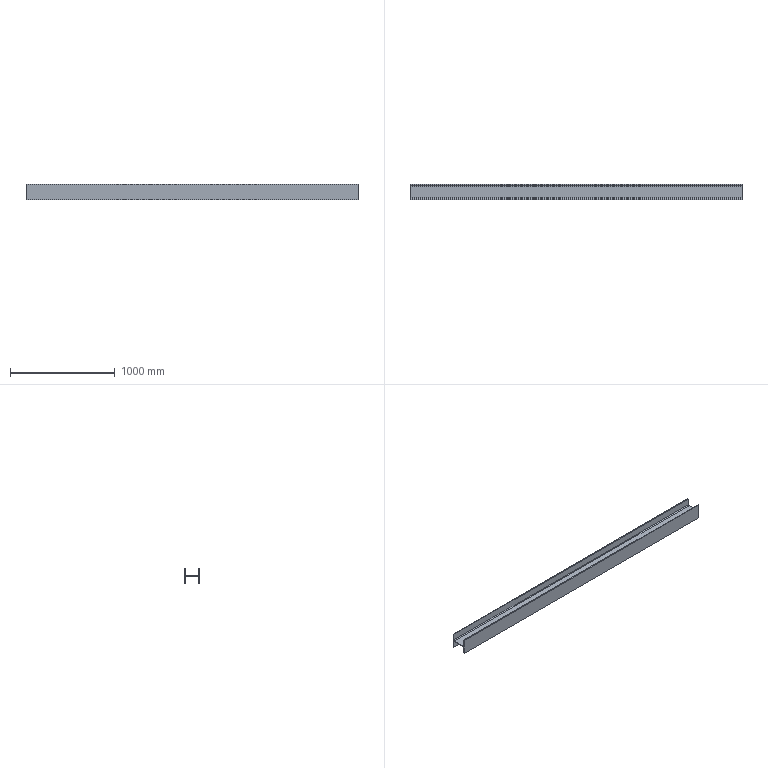Part | STEP file | 01-Cross beam H150X150_default<machining> | 1 solid | 18 faces | box 3170 x 150 x 150 mm | volume 12568854 mm3 | plane 14 | cylinder 4 | commonest cylinder face diameters 16 x4
STEP:
#1=CARTESIAN_POINT('',(0.,0.,0.));
#2=DIRECTION('',(0.,0.,1.));
#3=DIRECTION('',(1.,0.,0.));
#4=AXIS2_PLACEMENT_3D('',#1,#2,#3);
#5=CARTESIAN_POINT('',(0.,75.,75.));
#6=VERTEX_POINT('',#5);
#7=CARTESIAN_POINT('',(0.,65.,75.));
#8=VERTEX_POINT('',#7);
#9=CARTESIAN_POINT('',(0.,75.,75.));
#10=DIRECTION('',(0.,-1.,0.));
#11=VECTOR('',#10,1.);
#12=LINE('',#9,#11);
#13=CARTESIAN_POINT('',(3170.,75.,75.));
#14=DIRECTION('',(0.,0.,-1.));
#15=DIRECTION('',(0.,1.,0.));
#16=AXIS2_PLACEMENT_3D('',#13,#14,#15);
#17=PLANE('',#16);
#18=CARTESIAN_POINT('',(0.,-3170.));
#19=DIRECTION('',(-1.,0.));
#20=VECTOR('',#19,1.);
#21=LINE('',#18,#20);
#22=(GEOMETRIC_REPRESENTATION_CONTEXT(2)PARAMETRIC_REPRESENTATION_CONTEXT()REPRESENTATION_CONTEXT('',''));
#23=DEFINITIONAL_REPRESENTATION('',(#21),#22);
#24=PCURVE('',#17,#23);
#25=CARTESIAN_POINT('',(0.,57.,11.5));
#26=DIRECTION('',(1.,0.,0.));
#27=DIRECTION('',(0.,0.,-1.));
#28=AXIS2_PLACEMENT_3D('',#25,#26,#27);
#29=PLANE('',#28);
#30=CARTESIAN_POINT('',(-63.5,18.));
#31=DIRECTION('',(0.,-1.));
#32=VECTOR('',#31,1.);
#33=LINE('',#30,#32);
#34=(GEOMETRIC_REPRESENTATION_CONTEXT(2)PARAMETRIC_REPRESENTATION_CONTEXT()REPRESENTATION_CONTEXT('',''));
#35=DEFINITIONAL_REPRESENTATION('',(#33),#34);
#36=PCURVE('',#29,#35);
#37=SURFACE_CURVE('',#12,(#24,#36),.PCURVE_S1.);
#38=EDGE_CURVE('',#6,#8,#37,.T.);
#39=ORIENTED_EDGE('',*,*,#38,.T.);
#40=CARTESIAN_POINT('',(3170.,65.,75.));
#41=VERTEX_POINT('',#40);
#42=CARTESIAN_POINT('',(3170.,65.,75.));
#43=DIRECTION('',(-1.,0.,0.));
#44=VECTOR('',#43,1.);
#45=LINE('',#42,#44);
#46=CARTESIAN_POINT('',(-10.,0.));
#47=DIRECTION('',(0.,-1.));
#48=VECTOR('',#47,1.);
#49=LINE('',#46,#48);
#50=(GEOMETRIC_REPRESENTATION_CONTEXT(2)PARAMETRIC_REPRESENTATION_CONTEXT()REPRESENTATION_CONTEXT('',''));
#51=DEFINITIONAL_REPRESENTATION('',(#49),#50);
#52=PCURVE('',#17,#51);
#53=CARTESIAN_POINT('',(3170.,65.,75.));
#54=DIRECTION('',(0.,1.,0.));
#55=DIRECTION('',(0.,0.,1.));
#56=AXIS2_PLACEMENT_3D('',#53,#54,#55);
#57=PLANE('',#56);
#58=CARTESIAN_POINT('',(0.,0.));
#59=DIRECTION('',(0.,-1.));
#60=VECTOR('',#59,1.);
#61=LINE('',#58,#60);
#62=(GEOMETRIC_REPRESENTATION_CONTEXT(2)PARAMETRIC_REPRESENTATION_CONTEXT()REPRESENTATION_CONTEXT('',''));
#63=DEFINITIONAL_REPRESENTATION('',(#61),#62);
#64=PCURVE('',#57,#63);
#65=SURFACE_CURVE('',#45,(#52,#64),.PCURVE_S1.);
#66=EDGE_CURVE('',#41,#8,#65,.T.);
#67=ORIENTED_EDGE('',*,*,#66,.F.);
#68=CARTESIAN_POINT('',(3170.,75.,75.));
#69=VERTEX_POINT('',#68);
#70=CARTESIAN_POINT('',(3170.,75.,75.));
#71=DIRECTION('',(0.,-1.,0.));
#72=VECTOR('',#71,1.);
#73=LINE('',#70,#72);
#74=CARTESIAN_POINT('',(0.,0.));
#75=DIRECTION('',(-1.,0.));
#76=VECTOR('',#75,1.);
#77=LINE('',#74,#76);
#78=(GEOMETRIC_REPRESENTATION_CONTEXT(2)PARAMETRIC_REPRESENTATION_CONTEXT()REPRESENTATION_CONTEXT('',''));
#79=DEFINITIONAL_REPRESENTATION('',(#77),#78);
#80=PCURVE('',#17,#79);
#81=CARTESIAN_POINT('',(3170.,57.,11.5));
#82=DIRECTION('',(1.,0.,0.));
#83=DIRECTION('',(0.,0.,-1.));
#84=AXIS2_PLACEMENT_3D('',#81,#82,#83);
#85=PLANE('',#84);
#86=CARTESIAN_POINT('',(-63.5,18.));
#87=DIRECTION('',(0.,-1.));
#88=VECTOR('',#87,1.);
#89=LINE('',#86,#88);
#90=(GEOMETRIC_REPRESENTATION_CONTEXT(2)PARAMETRIC_REPRESENTATION_CONTEXT()REPRESENTATION_CONTEXT('',''));
#91=DEFINITIONAL_REPRESENTATION('',(#89),#90);
#92=PCURVE('',#85,#91);
#93=SURFACE_CURVE('',#73,(#80,#92),.PCURVE_S1.);
#94=EDGE_CURVE('',#69,#41,#93,.T.);
#95=ORIENTED_EDGE('',*,*,#94,.F.);
#96=CARTESIAN_POINT('',(3170.,75.,75.));
#97=DIRECTION('',(-1.,0.,0.));
#98=VECTOR('',#97,1.);
#99=LINE('',#96,#98);
#100=CARTESIAN_POINT('',(0.,0.));
#101=DIRECTION('',(0.,-1.));
#102=VECTOR('',#101,1.);
#103=LINE('',#100,#102);
#104=(GEOMETRIC_REPRESENTATION_CONTEXT(2)PARAMETRIC_REPRESENTATION_CONTEXT()REPRESENTATION_CONTEXT('',''));
#105=DEFINITIONAL_REPRESENTATION('',(#103),#104);
#106=PCURVE('',#17,#105);
#107=CARTESIAN_POINT('',(3170.,75.,-75.));
#108=DIRECTION('',(0.,-1.,0.));
#109=DIRECTION('',(0.,0.,-1.));
#110=AXIS2_PLACEMENT_3D('',#107,#108,#109);
#111=PLANE('',#110);
#112=CARTESIAN_POINT('',(-150.,0.));
#113=DIRECTION('',(0.,-1.));
#114=VECTOR('',#113,1.);
#115=LINE('',#112,#114);
#116=(GEOMETRIC_REPRESENTATION_CONTEXT(2)PARAMETRIC_REPRESENTATION_CONTEXT()REPRESENTATION_CONTEXT('',''));
#117=DEFINITIONAL_REPRESENTATION('',(#115),#116);
#118=PCURVE('',#111,#117);
#119=SURFACE_CURVE('',#99,(#106,#118),.PCURVE_S1.);
#120=EDGE_CURVE('',#69,#6,#119,.T.);
#121=ORIENTED_EDGE('',*,*,#120,.T.);
#122=EDGE_LOOP('',(#39,#67,#95,#121));
#123=FACE_BOUND('',#122,.T.);
#124=ADVANCED_FACE('',(#123),#17,.F.);
#125=CARTESIAN_POINT('',(0.,65.,11.5));
#126=VERTEX_POINT('',#125);
#127=CARTESIAN_POINT('',(0.,65.,75.));
#128=DIRECTION('',(0.,0.,-1.));
#129=VECTOR('',#128,1.);
#130=LINE('',#127,#129);
#131=CARTESIAN_POINT('',(0.,-3170.));
#132=DIRECTION('',(-1.,0.));
#133=VECTOR('',#132,1.);
#134=LINE('',#131,#133);
#135=(GEOMETRIC_REPRESENTATION_CONTEXT(2)PARAMETRIC_REPRESENTATION_CONTEXT()REPRESENTATION_CONTEXT('',''));
#136=DEFINITIONAL_REPRESENTATION('',(#134),#135);
#137=PCURVE('',#57,#136);
#138=CARTESIAN_POINT('',(-63.5,8.));
#139=DIRECTION('',(1.,0.));
#140=VECTOR('',#139,1.);
#141=LINE('',#138,#140);
#142=(GEOMETRIC_REPRESENTATION_CONTEXT(2)PARAMETRIC_REPRESENTATION_CONTEXT()REPRESENTATION_CONTEXT('',''));
#143=DEFINITIONAL_REPRESENTATION('',(#141),#142);
#144=PCURVE('',#29,#143);
#145=SURFACE_CURVE('',#130,(#137,#144),.PCURVE_S1.);
#146=EDGE_CURVE('',#8,#126,#145,.T.);
#147=ORIENTED_EDGE('',*,*,#146,.T.);
#148=CARTESIAN_POINT('',(3170.,65.,11.5));
#149=VERTEX_POINT('',#148);
#150=CARTESIAN_POINT('',(3170.,65.,11.5));
#151=DIRECTION('',(-1.,0.,0.));
#152=VECTOR('',#151,1.);
#153=LINE('',#150,#152);
#154=CARTESIAN_POINT('',(-63.5,0.));
#155=DIRECTION('',(0.,-1.));
#156=VECTOR('',#155,1.);
#157=LINE('',#154,#156);
#158=(GEOMETRIC_REPRESENTATION_CONTEXT(2)PARAMETRIC_REPRESENTATION_CONTEXT()REPRESENTATION_CONTEXT('',''));
#159=DEFINITIONAL_REPRESENTATION('',(#157),#158);
#160=PCURVE('',#57,#159);
#161=CARTESIAN_POINT('',(3170.,57.,11.5));
#162=DIRECTION('',(-1.,0.,0.));
#163=DIRECTION('',(0.,0.,1.));
#164=AXIS2_PLACEMENT_3D('',#161,#162,#163);
#165=CYLINDRICAL_SURFACE('',#164,8.);
#166=CARTESIAN_POINT('',(1.571,0.));
#167=DIRECTION('',(0.,1.));
#168=VECTOR('',#167,1.);
#169=LINE('',#166,#168);
#170=(GEOMETRIC_REPRESENTATION_CONTEXT(2)PARAMETRIC_REPRESENTATION_CONTEXT()REPRESENTATION_CONTEXT('',''));
#171=DEFINITIONAL_REPRESENTATION('',(#169),#170);
#172=PCURVE('',#165,#171);
#173=SURFACE_CURVE('',#153,(#160,#172),.PCURVE_S1.);
#174=EDGE_CURVE('',#149,#126,#173,.T.);
#175=ORIENTED_EDGE('',*,*,#174,.F.);
#176=CARTESIAN_POINT('',(3170.,65.,75.));
#177=DIRECTION('',(0.,0.,-1.));
#178=VECTOR('',#177,1.);
#179=LINE('',#176,#178);
#180=CARTESIAN_POINT('',(0.,0.));
#181=DIRECTION('',(-1.,0.));
#182=VECTOR('',#181,1.);
#183=LINE('',#180,#182);
#184=(GEOMETRIC_REPRESENTATION_CONTEXT(2)PARAMETRIC_REPRESENTATION_CONTEXT()REPRESENTATION_CONTEXT('',''));
#185=DEFINITIONAL_REPRESENTATION('',(#183),#184);
#186=PCURVE('',#57,#185);
#187=CARTESIAN_POINT('',(-63.5,8.));
#188=DIRECTION('',(1.,0.));
#189=VECTOR('',#188,1.);
#190=LINE('',#187,#189);
#191=(GEOMETRIC_REPRESENTATION_CONTEXT(2)PARAMETRIC_REPRESENTATION_CONTEXT()REPRESENTATION_CONTEXT('',''));
#192=DEFINITIONAL_REPRESENTATION('',(#190),#191);
#193=PCURVE('',#85,#192);
#194=SURFACE_CURVE('',#179,(#186,#193),.PCURVE_S1.);
#195=EDGE_CURVE('',#41,#149,#194,.T.);
#196=ORIENTED_EDGE('',*,*,#195,.F.);
#197=ORIENTED_EDGE('',*,*,#66,.T.);
#198=EDGE_LOOP('',(#147,#175,#196,#197));
#199=FACE_BOUND('',#198,.T.);
#200=ADVANCED_FACE('',(#199),#57,.F.);
#201=ORIENTED_EDGE('',*,*,#174,.F.);
#202=CARTESIAN_POINT('',(3170.,57.,3.5));
#203=VERTEX_POINT('',#202);
#204=CARTESIAN_POINT('',(3170.,57.,11.5));
#205=DIRECTION('',(-1.,0.,0.));
#206=DIRECTION('',(0.,0.,-1.));
#207=AXIS2_PLACEMENT_3D('',#204,#205,#206);
#208=CIRCLE('',#207,8.);
#209=CARTESIAN_POINT('',(-3.142,0.));
#210=DIRECTION('',(1.,0.));
#211=VECTOR('',#210,1.);
#212=LINE('',#209,#211);
#213=(GEOMETRIC_REPRESENTATION_CONTEXT(2)PARAMETRIC_REPRESENTATION_CONTEXT()REPRESENTATION_CONTEXT('',''));
#214=DEFINITIONAL_REPRESENTATION('',(#212),#213);
#215=PCURVE('',#165,#214);
#216=CARTESIAN_POINT('',(8.,0.));
#217=CARTESIAN_POINT('',(8.,-13.856));
#218=CARTESIAN_POINT('',(-4.,-6.928));
#219=CARTESIAN_POINT('',(-16.,0.));
#220=CARTESIAN_POINT('',(-4.,6.928));
#221=CARTESIAN_POINT('',(8.,13.856));
#222=CARTESIAN_POINT('',(8.,0.));
#223=(BOUNDED_CURVE()B_SPLINE_CURVE(2,(#216,#217,#218,#219,#220,#221,#222),.UNSPECIFIED.,.T.,.F.)B_SPLINE_CURVE_WITH_KNOTS((1,2,2,2,2,1),(-2.094,0.,2.094,4.189,6.283,8.378),.UNSPECIFIED.)CURVE()GEOMETRIC_REPRESENTATION_ITEM()RATIONAL_B_SPLINE_CURVE((1.,0.5,1.,0.5,1.,0.5,1.))REPRESENTATION_ITEM(''));
#224=(GEOMETRIC_REPRESENTATION_CONTEXT(2)PARAMETRIC_REPRESENTATION_CONTEXT()REPRESENTATION_CONTEXT('',''));
#225=DEFINITIONAL_REPRESENTATION('',(#223),#224);
#226=PCURVE('',#85,#225);
#227=SURFACE_CURVE('',#208,(#215,#226),.PCURVE_S1.);
#228=EDGE_CURVE('',#149,#203,#227,.T.);
#229=ORIENTED_EDGE('',*,*,#228,.T.);
#230=CARTESIAN_POINT('',(0.,57.,3.5));
#231=VERTEX_POINT('',#230);
#232=CARTESIAN_POINT('',(3170.,57.,3.5));
#233=DIRECTION('',(-1.,0.,0.));
#234=VECTOR('',#233,1.);
#235=LINE('',#232,#234);
#236=CARTESIAN_POINT('',(3.142,0.));
#237=DIRECTION('',(0.,1.));
#238=VECTOR('',#237,1.);
#239=LINE('',#236,#238);
#240=(GEOMETRIC_REPRESENTATION_CONTEXT(2)PARAMETRIC_REPRESENTATION_CONTEXT()REPRESENTATION_CONTEXT('',''));
#241=DEFINITIONAL_REPRESENTATION('',(#239),#240);
#242=PCURVE('',#165,#241);
#243=CARTESIAN_POINT('',(3170.,57.,3.5));
#244=DIRECTION('',(0.,0.,-1.));
#245=DIRECTION('',(-1.,0.,0.));
#246=AXIS2_PLACEMENT_3D('',#243,#244,#245);
#247=PLANE('',#246);
#248=CARTESIAN_POINT('',(0.,0.));
#249=DIRECTION('',(1.,0.));
#250=VECTOR('',#249,1.);
#251=LINE('',#248,#250);
#252=(GEOMETRIC_REPRESENTATION_CONTEXT(2)PARAMETRIC_REPRESENTATION_CONTEXT()REPRESENTATION_CONTEXT('',''));
#253=DEFINITIONAL_REPRESENTATION('',(#251),#252);
#254=PCURVE('',#247,#253);
#255=SURFACE_CURVE('',#235,(#242,#254),.PCURVE_S1.);
#256=EDGE_CURVE('',#203,#231,#255,.T.);
#257=ORIENTED_EDGE('',*,*,#256,.T.);
#258=CARTESIAN_POINT('',(0.,57.,11.5));
#259=DIRECTION('',(-1.,0.,0.));
#260=DIRECTION('',(0.,0.,-1.));
#261=AXIS2_PLACEMENT_3D('',#258,#259,#260);
#262=CIRCLE('',#261,8.);
#263=CARTESIAN_POINT('',(-3.142,3170.));
#264=DIRECTION('',(1.,0.));
#265=VECTOR('',#264,1.);
#266=LINE('',#263,#265);
#267=(GEOMETRIC_REPRESENTATION_CONTEXT(2)PARAMETRIC_REPRESENTATION_CONTEXT()REPRESENTATION_CONTEXT('',''));
#268=DEFINITIONAL_REPRESENTATION('',(#266),#267);
#269=PCURVE('',#165,#268);
#270=CARTESIAN_POINT('',(8.,0.));
#271=CARTESIAN_POINT('',(8.,-13.856));
#272=CARTESIAN_POINT('',(-4.,-6.928));
#273=CARTESIAN_POINT('',(-16.,0.));
#274=CARTESIAN_POINT('',(-4.,6.928));
#275=CARTESIAN_POINT('',(8.,13.856));
#276=CARTESIAN_POINT('',(8.,0.));
#277=(BOUNDED_CURVE()B_SPLINE_CURVE(2,(#270,#271,#272,#273,#274,#275,#276),.UNSPECIFIED.,.T.,.F.)B_SPLINE_CURVE_WITH_KNOTS((1,2,2,2,2,1),(-2.094,0.,2.094,4.189,6.283,8.378),.UNSPECIFIED.)CURVE()GEOMETRIC_REPRESENTATION_ITEM()RATIONAL_B_SPLINE_CURVE((1.,0.5,1.,0.5,1.,0.5,1.))REPRESENTATION_ITEM(''));
#278=(GEOMETRIC_REPRESENTATION_CONTEXT(2)PARAMETRIC_REPRESENTATION_CONTEXT()REPRESENTATION_CONTEXT('',''));
#279=DEFINITIONAL_REPRESENTATION('',(#277),#278);
#280=PCURVE('',#29,#279);
#281=SURFACE_CURVE('',#262,(#269,#280),.PCURVE_S1.);
#282=EDGE_CURVE('',#126,#231,#281,.T.);
#283=ORIENTED_EDGE('',*,*,#282,.F.);
#284=EDGE_LOOP('',(#201,#229,#257,#283));
#285=FACE_BOUND('',#284,.F.);
#286=ADVANCED_FACE('',(#285),#165,.F.);
#287=CARTESIAN_POINT('',(0.,-57.,3.5));
#288=VERTEX_POINT('',#287);
#289=CARTESIAN_POINT('',(0.,57.,3.5));
#290=DIRECTION('',(0.,-1.,0.));
#291=VECTOR('',#290,1.);
#292=LINE('',#289,#291);
#293=CARTESIAN_POINT('',(3170.,0.));
#294=DIRECTION('',(0.,-1.));
#295=VECTOR('',#294,1.);
#296=LINE('',#293,#295);
#297=(GEOMETRIC_REPRESENTATION_CONTEXT(2)PARAMETRIC_REPRESENTATION_CONTEXT()REPRESENTATION_CONTEXT('',''));
#298=DEFINITIONAL_REPRESENTATION('',(#296),#297);
#299=PCURVE('',#247,#298);
#300=CARTESIAN_POINT('',(8.,0.));
#301=DIRECTION('',(0.,-1.));
#302=VECTOR('',#301,1.);
#303=LINE('',#300,#302);
#304=(GEOMETRIC_REPRESENTATION_CONTEXT(2)PARAMETRIC_REPRESENTATION_CONTEXT()REPRESENTATION_CONTEXT('',''));
#305=DEFINITIONAL_REPRESENTATION('',(#303),#304);
#306=PCURVE('',#29,#305);
#307=SURFACE_CURVE('',#292,(#299,#306),.PCURVE_S1.);
#308=EDGE_CURVE('',#231,#288,#307,.T.);
#309=ORIENTED_EDGE('',*,*,#308,.T.);
#310=CARTESIAN_POINT('',(3170.,-57.,3.5));
#311=VERTEX_POINT('',#310);
#312=CARTESIAN_POINT('',(3170.,-57.,3.5));
#313=DIRECTION('',(-1.,0.,0.));
#314=VECTOR('',#313,1.);
#315=LINE('',#312,#314);
#316=CARTESIAN_POINT('',(0.,-114.));
#317=DIRECTION('',(1.,0.));
#318=VECTOR('',#317,1.);
#319=LINE('',#316,#318);
#320=(GEOMETRIC_REPRESENTATION_CONTEXT(2)PARAMETRIC_REPRESENTATION_CONTEXT()REPRESENTATION_CONTEXT('',''));
#321=DEFINITIONAL_REPRESENTATION('',(#319),#320);
#322=PCURVE('',#247,#321);
#323=CARTESIAN_POINT('',(3170.,-57.,11.5));
#324=DIRECTION('',(-1.,0.,0.));
#325=DIRECTION('',(0.,0.,1.));
#326=AXIS2_PLACEMENT_3D('',#323,#324,#325);
#327=CYLINDRICAL_SURFACE('',#326,8.);
#328=CARTESIAN_POINT('',(3.142,0.));
#329=DIRECTION('',(0.,1.));
#330=VECTOR('',#329,1.);
#331=LINE('',#328,#330);
#332=(GEOMETRIC_REPRESENTATION_CONTEXT(2)PARAMETRIC_REPRESENTATION_CONTEXT()REPRESENTATION_CONTEXT('',''));
#333=DEFINITIONAL_REPRESENTATION('',(#331),#332);
#334=PCURVE('',#327,#333);
#335=SURFACE_CURVE('',#315,(#322,#334),.PCURVE_S1.);
#336=EDGE_CURVE('',#311,#288,#335,.T.);
#337=ORIENTED_EDGE('',*,*,#336,.F.);
#338=CARTESIAN_POINT('',(3170.,57.,3.5));
#339=DIRECTION('',(0.,-1.,0.));
#340=VECTOR('',#339,1.);
#341=LINE('',#338,#340);
#342=CARTESIAN_POINT('',(0.,0.));
#343=DIRECTION('',(0.,-1.));
#344=VECTOR('',#343,1.);
#345=LINE('',#342,#344);
#346=(GEOMETRIC_REPRESENTATION_CONTEXT(2)PARAMETRIC_REPRESENTATION_CONTEXT()REPRESENTATION_CONTEXT('',''));
#347=DEFINITIONAL_REPRESENTATION('',(#345),#346);
#348=PCURVE('',#247,#347);
#349=CARTESIAN_POINT('',(8.,0.));
#350=DIRECTION('',(0.,-1.));
#351=VECTOR('',#350,1.);
#352=LINE('',#349,#351);
#353=(GEOMETRIC_REPRESENTATION_CONTEXT(2)PARAMETRIC_REPRESENTATION_CONTEXT()REPRESENTATION_CONTEXT('',''));
#354=DEFINITIONAL_REPRESENTATION('',(#352),#353);
#355=PCURVE('',#85,#354);
#356=SURFACE_CURVE('',#341,(#348,#355),.PCURVE_S1.);
#357=EDGE_CURVE('',#203,#311,#356,.T.);
#358=ORIENTED_EDGE('',*,*,#357,.F.);
#359=ORIENTED_EDGE('',*,*,#256,.T.);
#360=EDGE_LOOP('',(#309,#337,#358,#359));
#361=FACE_BOUND('',#360,.T.);
#362=ADVANCED_FACE('',(#361),#247,.F.);
#363=ORIENTED_EDGE('',*,*,#336,.F.);
#364=CARTESIAN_POINT('',(3170.,-65.,11.5));
#365=VERTEX_POINT('',#364);
#366=CARTESIAN_POINT('',(3170.,-57.,11.5));
#367=DIRECTION('',(-1.,0.,0.));
#368=DIRECTION('',(0.,0.,-1.));
#369=AXIS2_PLACEMENT_3D('',#366,#367,#368);
#370=CIRCLE('',#369,8.);
#371=CARTESIAN_POINT('',(3.142,0.));
#372=DIRECTION('',(1.,0.));
#373=VECTOR('',#372,1.);
#374=LINE('',#371,#373);
#375=(GEOMETRIC_REPRESENTATION_CONTEXT(2)PARAMETRIC_REPRESENTATION_CONTEXT()REPRESENTATION_CONTEXT('',''));
#376=DEFINITIONAL_REPRESENTATION('',(#374),#375);
#377=PCURVE('',#327,#376);
#378=CARTESIAN_POINT('',(8.,-114.));
#379=CARTESIAN_POINT('',(8.,-127.856));
#380=CARTESIAN_POINT('',(-4.,-120.928));
#381=CARTESIAN_POINT('',(-16.,-114.));
#382=CARTESIAN_POINT('',(-4.,-107.072));
#383=CARTESIAN_POINT('',(8.,-100.144));
#384=CARTESIAN_POINT('',(8.,-114.));
#385=(BOUNDED_CURVE()B_SPLINE_CURVE(2,(#378,#379,#380,#381,#382,#383,#384),.UNSPECIFIED.,.T.,.F.)B_SPLINE_CURVE_WITH_KNOTS((1,2,2,2,2,1),(-2.094,0.,2.094,4.189,6.283,8.378),.UNSPECIFIED.)CURVE()GEOMETRIC_REPRESENTATION_ITEM()RATIONAL_B_SPLINE_CURVE((1.,0.5,1.,0.5,1.,0.5,1.))REPRESENTATION_ITEM(''));
#386=(GEOMETRIC_REPRESENTATION_CONTEXT(2)PARAMETRIC_REPRESENTATION_CONTEXT()REPRESENTATION_CONTEXT('',''));
#387=DEFINITIONAL_REPRESENTATION('',(#385),#386);
#388=PCURVE('',#85,#387);
#389=SURFACE_CURVE('',#370,(#377,#388),.PCURVE_S1.);
#390=EDGE_CURVE('',#311,#365,#389,.T.);
#391=ORIENTED_EDGE('',*,*,#390,.T.);
#392=CARTESIAN_POINT('',(0.,-65.,11.5));
#393=VERTEX_POINT('',#392);
#394=CARTESIAN_POINT('',(3170.,-65.,11.5));
#395=DIRECTION('',(-1.,0.,0.));
#396=VECTOR('',#395,1.);
#397=LINE('',#394,#396);
#398=CARTESIAN_POINT('',(4.712,0.));
#399=DIRECTION('',(0.,1.));
#400=VECTOR('',#399,1.);
#401=LINE('',#398,#400);
#402=(GEOMETRIC_REPRESENTATION_CONTEXT(2)PARAMETRIC_REPRESENTATION_CONTEXT()REPRESENTATION_CONTEXT('',''));
#403=DEFINITIONAL_REPRESENTATION('',(#401),#402);
#404=PCURVE('',#327,#403);
#405=CARTESIAN_POINT('',(3170.,-65.,75.));
#406=DIRECTION('',(0.,-1.,0.));
#407=DIRECTION('',(0.,0.,-1.));
#408=AXIS2_PLACEMENT_3D('',#405,#406,#407);
#409=PLANE('',#408);
#410=CARTESIAN_POINT('',(63.5,0.));
#411=DIRECTION('',(0.,-1.));
#412=VECTOR('',#411,1.);
#413=LINE('',#410,#412);
#414=(GEOMETRIC_REPRESENTATION_CONTEXT(2)PARAMETRIC_REPRESENTATION_CONTEXT()REPRESENTATION_CONTEXT('',''));
#415=DEFINITIONAL_REPRESENTATION('',(#413),#414);
#416=PCURVE('',#409,#415);
#417=SURFACE_CURVE('',#397,(#404,#416),.PCURVE_S1.);
#418=EDGE_CURVE('',#365,#393,#417,.T.);
#419=ORIENTED_EDGE('',*,*,#418,.T.);
#420=CARTESIAN_POINT('',(0.,-57.,11.5));
#421=DIRECTION('',(-1.,0.,0.));
#422=DIRECTION('',(0.,0.,-1.));
#423=AXIS2_PLACEMENT_3D('',#420,#421,#422);
#424=CIRCLE('',#423,8.);
#425=CARTESIAN_POINT('',(3.142,3170.));
#426=DIRECTION('',(1.,0.));
#427=VECTOR('',#426,1.);
#428=LINE('',#425,#427);
#429=(GEOMETRIC_REPRESENTATION_CONTEXT(2)PARAMETRIC_REPRESENTATION_CONTEXT()REPRESENTATION_CONTEXT('',''));
#430=DEFINITIONAL_REPRESENTATION('',(#428),#429);
#431=PCURVE('',#327,#430);
#432=CARTESIAN_POINT('',(8.,-114.));
#433=CARTESIAN_POINT('',(8.,-127.856));
#434=CARTESIAN_POINT('',(-4.,-120.928));
#435=CARTESIAN_POINT('',(-16.,-114.));
#436=CARTESIAN_POINT('',(-4.,-107.072));
#437=CARTESIAN_POINT('',(8.,-100.144));
#438=CARTESIAN_POINT('',(8.,-114.));
#439=(BOUNDED_CURVE()B_SPLINE_CURVE(2,(#432,#433,#434,#435,#436,#437,#438),.UNSPECIFIED.,.T.,.F.)B_SPLINE_CURVE_WITH_KNOTS((1,2,2,2,2,1),(-2.094,0.,2.094,4.189,6.283,8.378),.UNSPECIFIED.)CURVE()GEOMETRIC_REPRESENTATION_ITEM()RATIONAL_B_SPLINE_CURVE((1.,0.5,1.,0.5,1.,0.5,1.))REPRESENTATION_ITEM(''));
#440=(GEOMETRIC_REPRESENTATION_CONTEXT(2)PARAMETRIC_REPRESENTATION_CONTEXT()REPRESENTATION_CONTEXT('',''));
#441=DEFINITIONAL_REPRESENTATION('',(#439),#440);
#442=PCURVE('',#29,#441);
#443=SURFACE_CURVE('',#424,(#431,#442),.PCURVE_S1.);
#444=EDGE_CURVE('',#288,#393,#443,.T.);
#445=ORIENTED_EDGE('',*,*,#444,.F.);
#446=EDGE_LOOP('',(#363,#391,#419,#445));
#447=FACE_BOUND('',#446,.F.);
#448=ADVANCED_FACE('',(#447),#327,.F.);
#449=CARTESIAN_POINT('',(0.,-65.,75.));
#450=VERTEX_POINT('',#449);
#451=CARTESIAN_POINT('',(0.,-65.,75.));
#452=DIRECTION('',(0.,0.,1.));
#453=VECTOR('',#452,1.);
#454=LINE('',#451,#453);
#455=CARTESIAN_POINT('',(0.,-3170.));
#456=DIRECTION('',(-1.,0.));
#457=VECTOR('',#456,1.);
#458=LINE('',#455,#457);
#459=(GEOMETRIC_REPRESENTATION_CONTEXT(2)PARAMETRIC_REPRESENTATION_CONTEXT()REPRESENTATION_CONTEXT('',''));
#460=DEFINITIONAL_REPRESENTATION('',(#458),#459);
#461=PCURVE('',#409,#460);
#462=CARTESIAN_POINT('',(-63.5,-122.));
#463=DIRECTION('',(-1.,0.));
#464=VECTOR('',#463,1.);
#465=LINE('',#462,#464);
#466=(GEOMETRIC_REPRESENTATION_CONTEXT(2)PARAMETRIC_REPRESENTATION_CONTEXT()REPRESENTATION_CONTEXT('',''));
#467=DEFINITIONAL_REPRESENTATION('',(#465),#466);
#468=PCURVE('',#29,#467);
#469=SURFACE_CURVE('',#454,(#461,#468),.PCURVE_S1.);
#470=EDGE_CURVE('',#393,#450,#469,.T.);
#471=ORIENTED_EDGE('',*,*,#470,.T.);
#472=CARTESIAN_POINT('',(3170.,-65.,75.));
#473=VERTEX_POINT('',#472);
#474=CARTESIAN_POINT('',(3170.,-65.,75.));
#475=DIRECTION('',(-1.,0.,0.));
#476=VECTOR('',#475,1.);
#477=LINE('',#474,#476);
#478=CARTESIAN_POINT('',(0.,0.));
#479=DIRECTION('',(0.,-1.));
#480=VECTOR('',#479,1.);
#481=LINE('',#478,#480);
#482=(GEOMETRIC_REPRESENTATION_CONTEXT(2)PARAMETRIC_REPRESENTATION_CONTEXT()REPRESENTATION_CONTEXT('',''));
#483=DEFINITIONAL_REPRESENTATION('',(#481),#482);
#484=PCURVE('',#409,#483);
#485=CARTESIAN_POINT('',(3170.,-75.,75.));
#486=DIRECTION('',(0.,0.,-1.));
#487=DIRECTION('',(0.,1.,0.));
#488=AXIS2_PLACEMENT_3D('',#485,#486,#487);
#489=PLANE('',#488);
#490=CARTESIAN_POINT('',(10.,0.));
#491=DIRECTION('',(0.,-1.));
#492=VECTOR('',#491,1.);
#493=LINE('',#490,#492);
#494=(GEOMETRIC_REPRESENTATION_CONTEXT(2)PARAMETRIC_REPRESENTATION_CONTEXT()REPRESENTATION_CONTEXT('',''));
#495=DEFINITIONAL_REPRESENTATION('',(#493),#494);
#496=PCURVE('',#489,#495);
#497=SURFACE_CURVE('',#477,(#484,#496),.PCURVE_S1.);
#498=EDGE_CURVE('',#473,#450,#497,.T.);
#499=ORIENTED_EDGE('',*,*,#498,.F.);
#500=CARTESIAN_POINT('',(3170.,-65.,75.));
#501=DIRECTION('',(0.,0.,1.));
#502=VECTOR('',#501,1.);
#503=LINE('',#500,#502);
#504=CARTESIAN_POINT('',(0.,0.));
#505=DIRECTION('',(-1.,0.));
#506=VECTOR('',#505,1.);
#507=LINE('',#504,#506);
#508=(GEOMETRIC_REPRESENTATION_CONTEXT(2)PARAMETRIC_REPRESENTATION_CONTEXT()REPRESENTATION_CONTEXT('',''));
#509=DEFINITIONAL_REPRESENTATION('',(#507),#508);
#510=PCURVE('',#409,#509);
#511=CARTESIAN_POINT('',(-63.5,-122.));
#512=DIRECTION('',(-1.,0.));
#513=VECTOR('',#512,1.);
#514=LINE('',#511,#513);
#515=(GEOMETRIC_REPRESENTATION_CONTEXT(2)PARAMETRIC_REPRESENTATION_CONTEXT()REPRESENTATION_CONTEXT('',''));
#516=DEFINITIONAL_REPRESENTATION('',(#514),#515);
#517=PCURVE('',#85,#516);
#518=SURFACE_CURVE('',#503,(#510,#517),.PCURVE_S1.);
#519=EDGE_CURVE('',#365,#473,#518,.T.);
#520=ORIENTED_EDGE('',*,*,#519,.F.);
#521=ORIENTED_EDGE('',*,*,#418,.T.);
#522=EDGE_LOOP('',(#471,#499,#520,#521));
#523=FACE_BOUND('',#522,.T.);
#524=ADVANCED_FACE('',(#523),#409,.F.);
#525=CARTESIAN_POINT('',(0.,-75.,75.));
#526=VERTEX_POINT('',#525);
#527=CARTESIAN_POINT('',(0.,-75.,75.));
#528=DIRECTION('',(0.,-1.,0.));
#529=VECTOR('',#528,1.);
#530=LINE('',#527,#529);
#531=CARTESIAN_POINT('',(0.,-3170.));
#532=DIRECTION('',(-1.,0.));
#533=VECTOR('',#532,1.);
#534=LINE('',#531,#533);
#535=(GEOMETRIC_REPRESENTATION_CONTEXT(2)PARAMETRIC_REPRESENTATION_CONTEXT()REPRESENTATION_CONTEXT('',''));
#536=DEFINITIONAL_REPRESENTATION('',(#534),#535);
#537=PCURVE('',#489,#536);
#538=CARTESIAN_POINT('',(-63.5,-132.));
#539=DIRECTION('',(0.,-1.));
#540=VECTOR('',#539,1.);
#541=LINE('',#538,#540);
#542=(GEOMETRIC_REPRESENTATION_CONTEXT(2)PARAMETRIC_REPRESENTATION_CONTEXT()REPRESENTATION_CONTEXT('',''));
#543=DEFINITIONAL_REPRESENTATION('',(#541),#542);
#544=PCURVE('',#29,#543);
#545=SURFACE_CURVE('',#530,(#537,#544),.PCURVE_S1.);
#546=EDGE_CURVE('',#450,#526,#545,.T.);
#547=ORIENTED_EDGE('',*,*,#546,.T.);
#548=CARTESIAN_POINT('',(3170.,-75.,75.));
#549=VERTEX_POINT('',#548);
#550=CARTESIAN_POINT('',(3170.,-75.,75.));
#551=DIRECTION('',(-1.,0.,0.));
#552=VECTOR('',#551,1.);
#553=LINE('',#550,#552);
#554=CARTESIAN_POINT('',(0.,0.));
#555=DIRECTION('',(0.,-1.));
#556=VECTOR('',#555,1.);
#557=LINE('',#554,#556);
#558=(GEOMETRIC_REPRESENTATION_CONTEXT(2)PARAMETRIC_REPRESENTATION_CONTEXT()REPRESENTATION_CONTEXT('',''));
#559=DEFINITIONAL_REPRESENTATION('',(#557),#558);
#560=PCURVE('',#489,#559);
#561=CARTESIAN_POINT('',(3170.,-75.,-75.));
#562=DIRECTION('',(0.,1.,0.));
#563=DIRECTION('',(0.,0.,1.));
#564=AXIS2_PLACEMENT_3D('',#561,#562,#563);
#565=PLANE('',#564);
#566=CARTESIAN_POINT('',(150.,0.));
#567=DIRECTION('',(0.,-1.));
#568=VECTOR('',#567,1.);
#569=LINE('',#566,#568);
#570=(GEOMETRIC_REPRESENTATION_CONTEXT(2)PARAMETRIC_REPRESENTATION_CONTEXT()REPRESENTATION_CONTEXT('',''));
#571=DEFINITIONAL_REPRESENTATION('',(#569),#570);
#572=PCURVE('',#565,#571);
#573=SURFACE_CURVE('',#553,(#560,#572),.PCURVE_S1.);
#574=EDGE_CURVE('',#549,#526,#573,.T.);
#575=ORIENTED_EDGE('',*,*,#574,.F.);
#576=CARTESIAN_POINT('',(3170.,-75.,75.));
#577=DIRECTION('',(0.,-1.,0.));
#578=VECTOR('',#577,1.);
#579=LINE('',#576,#578);
#580=CARTESIAN_POINT('',(0.,0.));
#581=DIRECTION('',(-1.,0.));
#582=VECTOR('',#581,1.);
#583=LINE('',#580,#582);
#584=(GEOMETRIC_REPRESENTATION_CONTEXT(2)PARAMETRIC_REPRESENTATION_CONTEXT()REPRESENTATION_CONTEXT('',''));
#585=DEFINITIONAL_REPRESENTATION('',(#583),#584);
#586=PCURVE('',#489,#585);
#587=CARTESIAN_POINT('',(-63.5,-132.));
#588=DIRECTION('',(0.,-1.));
#589=VECTOR('',#588,1.);
#590=LINE('',#587,#589);
#591=(GEOMETRIC_REPRESENTATION_CONTEXT(2)PARAMETRIC_REPRESENTATION_CONTEXT()REPRESENTATION_CONTEXT('',''));
#592=DEFINITIONAL_REPRESENTATION('',(#590),#591);
#593=PCURVE('',#85,#592);
#594=SURFACE_CURVE('',#579,(#586,#593),.PCURVE_S1.);
#595=EDGE_CURVE('',#473,#549,#594,.T.);
#596=ORIENTED_EDGE('',*,*,#595,.F.);
#597=ORIENTED_EDGE('',*,*,#498,.T.);
#598=EDGE_LOOP('',(#547,#575,#596,#597));
#599=FACE_BOUND('',#598,.T.);
#600=ADVANCED_FACE('',(#599),#489,.F.);
#601=CARTESIAN_POINT('',(0.,-75.,-75.));
#602=VERTEX_POINT('',#601);
#603=CARTESIAN_POINT('',(0.,-75.,-75.));
#604=DIRECTION('',(0.,0.,-1.));
#605=VECTOR('',#604,1.);
#606=LINE('',#603,#605);
#607=CARTESIAN_POINT('',(0.,-3170.));
#608=DIRECTION('',(-1.,0.));
#609=VECTOR('',#608,1.);
#610=LINE('',#607,#609);
#611=(GEOMETRIC_REPRESENTATION_CONTEXT(2)PARAMETRIC_REPRESENTATION_CONTEXT()REPRESENTATION_CONTEXT('',''));
#612=DEFINITIONAL_REPRESENTATION('',(#610),#611);
#613=PCURVE('',#565,#612);
#614=CARTESIAN_POINT('',(86.5,-132.));
#615=DIRECTION('',(1.,0.));
#616=VECTOR('',#615,1.);
#617=LINE('',#614,#616);
#618=(GEOMETRIC_REPRESENTATION_CONTEXT(2)PARAMETRIC_REPRESENTATION_CONTEXT()REPRESENTATION_CONTEXT('',''));
#619=DEFINITIONAL_REPRESENTATION('',(#617),#618);
#620=PCURVE('',#29,#619);
#621=SURFACE_CURVE('',#606,(#613,#620),.PCURVE_S1.);
#622=EDGE_CURVE('',#526,#602,#621,.T.);
#623=ORIENTED_EDGE('',*,*,#622,.T.);
#624=CARTESIAN_POINT('',(3170.,-75.,-75.));
#625=VERTEX_POINT('',#624);
#626=CARTESIAN_POINT('',(3170.,-75.,-75.));
#627=DIRECTION('',(-1.,0.,0.));
#628=VECTOR('',#627,1.);
#629=LINE('',#626,#628);
#630=CARTESIAN_POINT('',(0.,0.));
#631=DIRECTION('',(0.,-1.));
#632=VECTOR('',#631,1.);
#633=LINE('',#630,#632);
#634=(GEOMETRIC_REPRESENTATION_CONTEXT(2)PARAMETRIC_REPRESENTATION_CONTEXT()REPRESENTATION_CONTEXT('',''));
#635=DEFINITIONAL_REPRESENTATION('',(#633),#634);
#636=PCURVE('',#565,#635);
#637=CARTESIAN_POINT('',(3170.,-75.,-75.));
#638=DIRECTION('',(0.,0.,1.));
#639=DIRECTION('',(0.,-1.,0.));
#640=AXIS2_PLACEMENT_3D('',#637,#638,#639);
#641=PLANE('',#640);
#642=CARTESIAN_POINT('',(0.,0.));
#643=DIRECTION('',(0.,-1.));
#644=VECTOR('',#643,1.);
#645=LINE('',#642,#644);
#646=(GEOMETRIC_REPRESENTATION_CONTEXT(2)PARAMETRIC_REPRESENTATION_CONTEXT()REPRESENTATION_CONTEXT('',''));
#647=DEFINITIONAL_REPRESENTATION('',(#645),#646);
#648=PCURVE('',#641,#647);
#649=SURFACE_CURVE('',#629,(#636,#648),.PCURVE_S1.);
#650=EDGE_CURVE('',#625,#602,#649,.T.);
#651=ORIENTED_EDGE('',*,*,#650,.F.);
#652=CARTESIAN_POINT('',(3170.,-75.,-75.));
#653=DIRECTION('',(0.,0.,-1.));
#654=VECTOR('',#653,1.);
#655=LINE('',#652,#654);
#656=CARTESIAN_POINT('',(0.,0.));
#657=DIRECTION('',(-1.,0.));
#658=VECTOR('',#657,1.);
#659=LINE('',#656,#658);
#660=(GEOMETRIC_REPRESENTATION_CONTEXT(2)PARAMETRIC_REPRESENTATION_CONTEXT()REPRESENTATION_CONTEXT('',''));
#661=DEFINITIONAL_REPRESENTATION('',(#659),#660);
#662=PCURVE('',#565,#661);
#663=CARTESIAN_POINT('',(86.5,-132.));
#664=DIRECTION('',(1.,0.));
#665=VECTOR('',#664,1.);
#666=LINE('',#663,#665);
#667=(GEOMETRIC_REPRESENTATION_CONTEXT(2)PARAMETRIC_REPRESENTATION_CONTEXT()REPRESENTATION_CONTEXT('',''));
#668=DEFINITIONAL_REPRESENTATION('',(#666),#667);
#669=PCURVE('',#85,#668);
#670=SURFACE_CURVE('',#655,(#662,#669),.PCURVE_S1.);
#671=EDGE_CURVE('',#549,#625,#670,.T.);
#672=ORIENTED_EDGE('',*,*,#671,.F.);
#673=ORIENTED_EDGE('',*,*,#574,.T.);
#674=EDGE_LOOP('',(#623,#651,#672,#673));
#675=FACE_BOUND('',#674,.T.);
#676=ADVANCED_FACE('',(#675),#565,.F.);
#677=CARTESIAN_POINT('',(0.,-65.,-75.));
#678=VERTEX_POINT('',#677);
#679=CARTESIAN_POINT('',(0.,-75.,-75.));
#680=DIRECTION('',(0.,1.,0.));
#681=VECTOR('',#680,1.);
#682=LINE('',#679,#681);
#683=CARTESIAN_POINT('',(0.,-3170.));
#684=DIRECTION('',(-1.,0.));
#685=VECTOR('',#684,1.);
#686=LINE('',#683,#685);
#687=(GEOMETRIC_REPRESENTATION_CONTEXT(2)PARAMETRIC_REPRESENTATION_CONTEXT()REPRESENTATION_CONTEXT('',''));
#688=DEFINITIONAL_REPRESENTATION('',(#686),#687);
#689=PCURVE('',#641,#688);
#690=CARTESIAN_POINT('',(86.5,-132.));
#691=DIRECTION('',(0.,1.));
#692=VECTOR('',#691,1.);
#693=LINE('',#690,#692);
#694=(GEOMETRIC_REPRESENTATION_CONTEXT(2)PARAMETRIC_REPRESENTATION_CONTEXT()REPRESENTATION_CONTEXT('',''));
#695=DEFINITIONAL_REPRESENTATION('',(#693),#694);
#696=PCURVE('',#29,#695);
#697=SURFACE_CURVE('',#682,(#689,#696),.PCURVE_S1.);
#698=EDGE_CURVE('',#602,#678,#697,.T.);
#699=ORIENTED_EDGE('',*,*,#698,.T.);
#700=CARTESIAN_POINT('',(3170.,-65.,-75.));
#701=VERTEX_POINT('',#700);
#702=CARTESIAN_POINT('',(3170.,-65.,-75.));
#703=DIRECTION('',(-1.,0.,0.));
#704=VECTOR('',#703,1.);
#705=LINE('',#702,#704);
#706=CARTESIAN_POINT('',(-10.,0.));
#707=DIRECTION('',(0.,-1.));
#708=VECTOR('',#707,1.);
#709=LINE('',#706,#708);
#710=(GEOMETRIC_REPRESENTATION_CONTEXT(2)PARAMETRIC_REPRESENTATION_CONTEXT()REPRESENTATION_CONTEXT('',''));
#711=DEFINITIONAL_REPRESENTATION('',(#709),#710);
#712=PCURVE('',#641,#711);
#713=CARTESIAN_POINT('',(3170.,-65.,-75.));
#714=DIRECTION('',(0.,-1.,0.));
#715=DIRECTION('',(0.,0.,-1.));
#716=AXIS2_PLACEMENT_3D('',#713,#714,#715);
#717=PLANE('',#716);
#718=CARTESIAN_POINT('',(0.,0.));
#719=DIRECTION('',(0.,-1.));
#720=VECTOR('',#719,1.);
#721=LINE('',#718,#720);
#722=(GEOMETRIC_REPRESENTATION_CONTEXT(2)PARAMETRIC_REPRESENTATION_CONTEXT()REPRESENTATION_CONTEXT('',''));
#723=DEFINITIONAL_REPRESENTATION('',(#721),#722);
#724=PCURVE('',#717,#723);
#725=SURFACE_CURVE('',#705,(#712,#724),.PCURVE_S1.);
#726=EDGE_CURVE('',#701,#678,#725,.T.);
#727=ORIENTED_EDGE('',*,*,#726,.F.);
#728=CARTESIAN_POINT('',(3170.,-75.,-75.));
#729=DIRECTION('',(0.,1.,0.));
#730=VECTOR('',#729,1.);
#731=LINE('',#728,#730);
#732=CARTESIAN_POINT('',(0.,0.));
#733=DIRECTION('',(-1.,0.));
#734=VECTOR('',#733,1.);
#735=LINE('',#732,#734);
#736=(GEOMETRIC_REPRESENTATION_CONTEXT(2)PARAMETRIC_REPRESENTATION_CONTEXT()REPRESENTATION_CONTEXT('',''));
#737=DEFINITIONAL_REPRESENTATION('',(#735),#736);
#738=PCURVE('',#641,#737);
#739=CARTESIAN_POINT('',(86.5,-132.));
#740=DIRECTION('',(0.,1.));
#741=VECTOR('',#740,1.);
#742=LINE('',#739,#741);
#743=(GEOMETRIC_REPRESENTATION_CONTEXT(2)PARAMETRIC_REPRESENTATION_CONTEXT()REPRESENTATION_CONTEXT('',''));
#744=DEFINITIONAL_REPRESENTATION('',(#742),#743);
#745=PCURVE('',#85,#744);
#746=SURFACE_CURVE('',#731,(#738,#745),.PCURVE_S1.);
#747=EDGE_CURVE('',#625,#701,#746,.T.);
#748=ORIENTED_EDGE('',*,*,#747,.F.);
#749=ORIENTED_EDGE('',*,*,#650,.T.);
#750=EDGE_LOOP('',(#699,#727,#748,#749));
#751=FACE_BOUND('',#750,.T.);
#752=ADVANCED_FACE('',(#751),#641,.F.);
#753=CARTESIAN_POINT('',(0.,-65.,-11.5));
#754=VERTEX_POINT('',#753);
#755=CARTESIAN_POINT('',(0.,-65.,-75.));
#756=DIRECTION('',(0.,0.,1.));
#757=VECTOR('',#756,1.);
#758=LINE('',#755,#757);
#759=CARTESIAN_POINT('',(0.,-3170.));
#760=DIRECTION('',(-1.,0.));
#761=VECTOR('',#760,1.);
#762=LINE('',#759,#761);
#763=(GEOMETRIC_REPRESENTATION_CONTEXT(2)PARAMETRIC_REPRESENTATION_CONTEXT()REPRESENTATION_CONTEXT('',''));
#764=DEFINITIONAL_REPRESENTATION('',(#762),#763);
#765=PCURVE('',#717,#764);
#766=CARTESIAN_POINT('',(86.5,-122.));
#767=DIRECTION('',(-1.,0.));
#768=VECTOR('',#767,1.);
#769=LINE('',#766,#768);
#770=(GEOMETRIC_REPRESENTATION_CONTEXT(2)PARAMETRIC_REPRESENTATION_CONTEXT()REPRESENTATION_CONTEXT('',''));
#771=DEFINITIONAL_REPRESENTATION('',(#769),#770);
#772=PCURVE('',#29,#771);
#773=SURFACE_CURVE('',#758,(#765,#772),.PCURVE_S1.);
#774=EDGE_CURVE('',#678,#754,#773,.T.);
#775=ORIENTED_EDGE('',*,*,#774,.T.);
#776=CARTESIAN_POINT('',(3170.,-65.,-11.5));
#777=VERTEX_POINT('',#776);
#778=CARTESIAN_POINT('',(3170.,-65.,-11.5));
#779=DIRECTION('',(-1.,0.,0.));
#780=VECTOR('',#779,1.);
#781=LINE('',#778,#780);
#782=CARTESIAN_POINT('',(-63.5,0.));
#783=DIRECTION('',(0.,-1.));
#784=VECTOR('',#783,1.);
#785=LINE('',#782,#784);
#786=(GEOMETRIC_REPRESENTATION_CONTEXT(2)PARAMETRIC_REPRESENTATION_CONTEXT()REPRESENTATION_CONTEXT('',''));
#787=DEFINITIONAL_REPRESENTATION('',(#785),#786);
#788=PCURVE('',#717,#787);
#789=CARTESIAN_POINT('',(3170.,-57.,-11.5));
#790=DIRECTION('',(-1.,0.,0.));
#791=DIRECTION('',(0.,0.,1.));
#792=AXIS2_PLACEMENT_3D('',#789,#790,#791);
#793=CYLINDRICAL_SURFACE('',#792,8.);
#794=CARTESIAN_POINT('',(4.712,0.));
#795=DIRECTION('',(0.,1.));
#796=VECTOR('',#795,1.);
#797=LINE('',#794,#796);
#798=(GEOMETRIC_REPRESENTATION_CONTEXT(2)PARAMETRIC_REPRESENTATION_CONTEXT()REPRESENTATION_CONTEXT('',''));
#799=DEFINITIONAL_REPRESENTATION('',(#797),#798);
#800=PCURVE('',#793,#799);
#801=SURFACE_CURVE('',#781,(#788,#800),.PCURVE_S1.);
#802=EDGE_CURVE('',#777,#754,#801,.T.);
#803=ORIENTED_EDGE('',*,*,#802,.F.);
#804=CARTESIAN_POINT('',(3170.,-65.,-75.));
#805=DIRECTION('',(0.,0.,1.));
#806=VECTOR('',#805,1.);
#807=LINE('',#804,#806);
#808=CARTESIAN_POINT('',(0.,0.));
#809=DIRECTION('',(-1.,0.));
#810=VECTOR('',#809,1.);
#811=LINE('',#808,#810);
#812=(GEOMETRIC_REPRESENTATION_CONTEXT(2)PARAMETRIC_REPRESENTATION_CONTEXT()REPRESENTATION_CONTEXT('',''));
#813=DEFINITIONAL_REPRESENTATION('',(#811),#812);
#814=PCURVE('',#717,#813);
#815=CARTESIAN_POINT('',(86.5,-122.));
#816=DIRECTION('',(-1.,0.));
#817=VECTOR('',#816,1.);
#818=LINE('',#815,#817);
#819=(GEOMETRIC_REPRESENTATION_CONTEXT(2)PARAMETRIC_REPRESENTATION_CONTEXT()REPRESENTATION_CONTEXT('',''));
#820=DEFINITIONAL_REPRESENTATION('',(#818),#819);
#821=PCURVE('',#85,#820);
#822=SURFACE_CURVE('',#807,(#814,#821),.PCURVE_S1.);
#823=EDGE_CURVE('',#701,#777,#822,.T.);
#824=ORIENTED_EDGE('',*,*,#823,.F.);
#825=ORIENTED_EDGE('',*,*,#726,.T.);
#826=EDGE_LOOP('',(#775,#803,#824,#825));
#827=FACE_BOUND('',#826,.T.);
#828=ADVANCED_FACE('',(#827),#717,.F.);
#829=ORIENTED_EDGE('',*,*,#802,.F.);
#830=CARTESIAN_POINT('',(3170.,-57.,-3.5));
#831=VERTEX_POINT('',#830);
#832=CARTESIAN_POINT('',(3170.,-57.,-11.5));
#833=DIRECTION('',(-1.,0.,0.));
#834=DIRECTION('',(0.,0.,1.));
#835=AXIS2_PLACEMENT_3D('',#832,#833,#834);
#836=CIRCLE('',#835,8.);
#837=CARTESIAN_POINT('',(0.,0.));
#838=DIRECTION('',(1.,0.));
#839=VECTOR('',#838,1.);
#840=LINE('',#837,#839);
#841=(GEOMETRIC_REPRESENTATION_CONTEXT(2)PARAMETRIC_REPRESENTATION_CONTEXT()REPRESENTATION_CONTEXT('',''));
#842=DEFINITIONAL_REPRESENTATION('',(#840),#841);
#843=PCURVE('',#793,#842);
#844=CARTESIAN_POINT('',(15.,-114.));
#845=CARTESIAN_POINT('',(15.,-100.144));
#846=CARTESIAN_POINT('',(27.,-107.072));
#847=CARTESIAN_POINT('',(39.,-114.));
#848=CARTESIAN_POINT('',(27.,-120.928));
#849=CARTESIAN_POINT('',(15.,-127.856));
#850=CARTESIAN_POINT('',(15.,-114.));
#851=(BOUNDED_CURVE()B_SPLINE_CURVE(2,(#844,#845,#846,#847,#848,#849,#850),.UNSPECIFIED.,.T.,.F.)B_SPLINE_CURVE_WITH_KNOTS((1,2,2,2,2,1),(-2.094,0.,2.094,4.189,6.283,8.378),.UNSPECIFIED.)CURVE()GEOMETRIC_REPRESENTATION_ITEM()RATIONAL_B_SPLINE_CURVE((1.,0.5,1.,0.5,1.,0.5,1.))REPRESENTATION_ITEM(''));
#852=(GEOMETRIC_REPRESENTATION_CONTEXT(2)PARAMETRIC_REPRESENTATION_CONTEXT()REPRESENTATION_CONTEXT('',''));
#853=DEFINITIONAL_REPRESENTATION('',(#851),#852);
#854=PCURVE('',#85,#853);
#855=SURFACE_CURVE('',#836,(#843,#854),.PCURVE_S1.);
#856=EDGE_CURVE('',#777,#831,#855,.T.);
#857=ORIENTED_EDGE('',*,*,#856,.T.);
#858=CARTESIAN_POINT('',(0.,-57.,-3.5));
#859=VERTEX_POINT('',#858);
#860=CARTESIAN_POINT('',(3170.,-57.,-3.5));
#861=DIRECTION('',(-1.,0.,0.));
#862=VECTOR('',#861,1.);
#863=LINE('',#860,#862);
#864=CARTESIAN_POINT('',(6.283,0.));
#865=DIRECTION('',(0.,1.));
#866=VECTOR('',#865,1.);
#867=LINE('',#864,#866);
#868=(GEOMETRIC_REPRESENTATION_CONTEXT(2)PARAMETRIC_REPRESENTATION_CONTEXT()REPRESENTATION_CONTEXT('',''));
#869=DEFINITIONAL_REPRESENTATION('',(#867),#868);
#870=PCURVE('',#793,#869);
#871=CARTESIAN_POINT('',(3170.,57.,-3.5));
#872=DIRECTION('',(0.,0.,1.));
#873=DIRECTION('',(1.,0.,0.));
#874=AXIS2_PLACEMENT_3D('',#871,#872,#873);
#875=PLANE('',#874);
#876=CARTESIAN_POINT('',(0.,-114.));
#877=DIRECTION('',(-1.,0.));
#878=VECTOR('',#877,1.);
#879=LINE('',#876,#878);
#880=(GEOMETRIC_REPRESENTATION_CONTEXT(2)PARAMETRIC_REPRESENTATION_CONTEXT()REPRESENTATION_CONTEXT('',''));
#881=DEFINITIONAL_REPRESENTATION('',(#879),#880);
#882=PCURVE('',#875,#881);
#883=SURFACE_CURVE('',#863,(#870,#882),.PCURVE_S1.);
#884=EDGE_CURVE('',#831,#859,#883,.T.);
#885=ORIENTED_EDGE('',*,*,#884,.T.);
#886=CARTESIAN_POINT('',(0.,-57.,-11.5));
#887=DIRECTION('',(-1.,0.,0.));
#888=DIRECTION('',(0.,0.,1.));
#889=AXIS2_PLACEMENT_3D('',#886,#887,#888);
#890=CIRCLE('',#889,8.);
#891=CARTESIAN_POINT('',(0.,3170.));
#892=DIRECTION('',(1.,0.));
#893=VECTOR('',#892,1.);
#894=LINE('',#891,#893);
#895=(GEOMETRIC_REPRESENTATION_CONTEXT(2)PARAMETRIC_REPRESENTATION_CONTEXT()REPRESENTATION_CONTEXT('',''));
#896=DEFINITIONAL_REPRESENTATION('',(#894),#895);
#897=PCURVE('',#793,#896);
#898=CARTESIAN_POINT('',(15.,-114.));
#899=CARTESIAN_POINT('',(15.,-100.144));
#900=CARTESIAN_POINT('',(27.,-107.072));
#901=CARTESIAN_POINT('',(39.,-114.));
#902=CARTESIAN_POINT('',(27.,-120.928));
#903=CARTESIAN_POINT('',(15.,-127.856));
#904=CARTESIAN_POINT('',(15.,-114.));
#905=(BOUNDED_CURVE()B_SPLINE_CURVE(2,(#898,#899,#900,#901,#902,#903,#904),.UNSPECIFIED.,.T.,.F.)B_SPLINE_CURVE_WITH_KNOTS((1,2,2,2,2,1),(-2.094,0.,2.094,4.189,6.283,8.378),.UNSPECIFIED.)CURVE()GEOMETRIC_REPRESENTATION_ITEM()RATIONAL_B_SPLINE_CURVE((1.,0.5,1.,0.5,1.,0.5,1.))REPRESENTATION_ITEM(''));
#906=(GEOMETRIC_REPRESENTATION_CONTEXT(2)PARAMETRIC_REPRESENTATION_CONTEXT()REPRESENTATION_CONTEXT('',''));
#907=DEFINITIONAL_REPRESENTATION('',(#905),#906);
#908=PCURVE('',#29,#907);
#909=SURFACE_CURVE('',#890,(#897,#908),.PCURVE_S1.);
#910=EDGE_CURVE('',#754,#859,#909,.T.);
#911=ORIENTED_EDGE('',*,*,#910,.F.);
#912=EDGE_LOOP('',(#829,#857,#885,#911));
#913=FACE_BOUND('',#912,.F.);
#914=ADVANCED_FACE('',(#913),#793,.F.);
#915=CARTESIAN_POINT('',(0.,57.,-3.5));
#916=VERTEX_POINT('',#915);
#917=CARTESIAN_POINT('',(0.,57.,-3.5));
#918=DIRECTION('',(0.,1.,0.));
#919=VECTOR('',#918,1.);
#920=LINE('',#917,#919);
#921=CARTESIAN_POINT('',(-3170.,0.));
#922=DIRECTION('',(0.,1.));
#923=VECTOR('',#922,1.);
#924=LINE('',#921,#923);
#925=(GEOMETRIC_REPRESENTATION_CONTEXT(2)PARAMETRIC_REPRESENTATION_CONTEXT()REPRESENTATION_CONTEXT('',''));
#926=DEFINITIONAL_REPRESENTATION('',(#924),#925);
#927=PCURVE('',#875,#926);
#928=CARTESIAN_POINT('',(15.,0.));
#929=DIRECTION('',(0.,1.));
#930=VECTOR('',#929,1.);
#931=LINE('',#928,#930);
#932=(GEOMETRIC_REPRESENTATION_CONTEXT(2)PARAMETRIC_REPRESENTATION_CONTEXT()REPRESENTATION_CONTEXT('',''));
#933=DEFINITIONAL_REPRESENTATION('',(#931),#932);
#934=PCURVE('',#29,#933);
#935=SURFACE_CURVE('',#920,(#927,#934),.PCURVE_S1.);
#936=EDGE_CURVE('',#859,#916,#935,.T.);
#937=ORIENTED_EDGE('',*,*,#936,.T.);
#938=CARTESIAN_POINT('',(3170.,57.,-3.5));
#939=VERTEX_POINT('',#938);
#940=CARTESIAN_POINT('',(3170.,57.,-3.5));
#941=DIRECTION('',(-1.,0.,0.));
#942=VECTOR('',#941,1.);
#943=LINE('',#940,#942);
#944=CARTESIAN_POINT('',(0.,0.));
#945=DIRECTION('',(-1.,0.));
#946=VECTOR('',#945,1.);
#947=LINE('',#944,#946);
#948=(GEOMETRIC_REPRESENTATION_CONTEXT(2)PARAMETRIC_REPRESENTATION_CONTEXT()REPRESENTATION_CONTEXT('',''));
#949=DEFINITIONAL_REPRESENTATION('',(#947),#948);
#950=PCURVE('',#875,#949);
#951=CARTESIAN_POINT('',(3170.,57.,-11.5));
#952=DIRECTION('',(-1.,0.,0.));
#953=DIRECTION('',(0.,0.,1.));
#954=AXIS2_PLACEMENT_3D('',#951,#952,#953);
#955=CYLINDRICAL_SURFACE('',#954,8.);
#956=CARTESIAN_POINT('',(0.,0.));
#957=DIRECTION('',(0.,1.));
#958=VECTOR('',#957,1.);
#959=LINE('',#956,#958);
#960=(GEOMETRIC_REPRESENTATION_CONTEXT(2)PARAMETRIC_REPRESENTATION_CONTEXT()REPRESENTATION_CONTEXT('',''));
#961=DEFINITIONAL_REPRESENTATION('',(#959),#960);
#962=PCURVE('',#955,#961);
#963=SURFACE_CURVE('',#943,(#950,#962),.PCURVE_S1.);
#964=EDGE_CURVE('',#939,#916,#963,.T.);
#965=ORIENTED_EDGE('',*,*,#964,.F.);
#966=CARTESIAN_POINT('',(3170.,57.,-3.5));
#967=DIRECTION('',(0.,1.,0.));
#968=VECTOR('',#967,1.);
#969=LINE('',#966,#968);
#970=CARTESIAN_POINT('',(0.,0.));
#971=DIRECTION('',(0.,1.));
#972=VECTOR('',#971,1.);
#973=LINE('',#970,#972);
#974=(GEOMETRIC_REPRESENTATION_CONTEXT(2)PARAMETRIC_REPRESENTATION_CONTEXT()REPRESENTATION_CONTEXT('',''));
#975=DEFINITIONAL_REPRESENTATION('',(#973),#974);
#976=PCURVE('',#875,#975);
#977=CARTESIAN_POINT('',(15.,0.));
#978=DIRECTION('',(0.,1.));
#979=VECTOR('',#978,1.);
#980=LINE('',#977,#979);
#981=(GEOMETRIC_REPRESENTATION_CONTEXT(2)PARAMETRIC_REPRESENTATION_CONTEXT()REPRESENTATION_CONTEXT('',''));
#982=DEFINITIONAL_REPRESENTATION('',(#980),#981);
#983=PCURVE('',#85,#982);
#984=SURFACE_CURVE('',#969,(#976,#983),.PCURVE_S1.);
#985=EDGE_CURVE('',#831,#939,#984,.T.);
#986=ORIENTED_EDGE('',*,*,#985,.F.);
#987=ORIENTED_EDGE('',*,*,#884,.T.);
#988=EDGE_LOOP('',(#937,#965,#986,#987));
#989=FACE_BOUND('',#988,.T.);
#990=ADVANCED_FACE('',(#989),#875,.F.);
#991=ORIENTED_EDGE('',*,*,#964,.F.);
#992=CARTESIAN_POINT('',(3170.,65.,-11.5));
#993=VERTEX_POINT('',#992);
#994=CARTESIAN_POINT('',(3170.,57.,-11.5));
#995=DIRECTION('',(-1.,0.,0.));
#996=DIRECTION('',(0.,0.,1.));
#997=AXIS2_PLACEMENT_3D('',#994,#995,#996);
#998=CIRCLE('',#997,8.);
#999=CARTESIAN_POINT('',(0.,0.));
#1000=DIRECTION('',(1.,0.));
#1001=VECTOR('',#1000,1.);
#1002=LINE('',#999,#1001);
#1003=(GEOMETRIC_REPRESENTATION_CONTEXT(2)PARAMETRIC_REPRESENTATION_CONTEXT()REPRESENTATION_CONTEXT('',''));
#1004=DEFINITIONAL_REPRESENTATION('',(#1002),#1003);
#1005=PCURVE('',#955,#1004);
#1006=CARTESIAN_POINT('',(15.,0.));
#1007=CARTESIAN_POINT('',(15.,13.856));
#1008=CARTESIAN_POINT('',(27.,6.928));
#1009=CARTESIAN_POINT('',(39.,0.));
#1010=CARTESIAN_POINT('',(27.,-6.928));
#1011=CARTESIAN_POINT('',(15.,-13.856));
#1012=CARTESIAN_POINT('',(15.,0.));
#1013=(BOUNDED_CURVE()B_SPLINE_CURVE(2,(#1006,#1007,#1008,#1009,#1010,#1011,#1012),.UNSPECIFIED.,.T.,.F.)B_SPLINE_CURVE_WITH_KNOTS((1,2,2,2,2,1),(-2.094,0.,2.094,4.189,6.283,8.378),.UNSPECIFIED.)CURVE()GEOMETRIC_REPRESENTATION_ITEM()RATIONAL_B_SPLINE_CURVE((1.,0.5,1.,0.5,1.,0.5,1.))REPRESENTATION_ITEM(''));
#1014=(GEOMETRIC_REPRESENTATION_CONTEXT(2)PARAMETRIC_REPRESENTATION_CONTEXT()REPRESENTATION_CONTEXT('',''));
#1015=DEFINITIONAL_REPRESENTATION('',(#1013),#1014);
#1016=PCURVE('',#85,#1015);
#1017=SURFACE_CURVE('',#998,(#1005,#1016),.PCURVE_S1.);
#1018=EDGE_CURVE('',#939,#993,#1017,.T.);
#1019=ORIENTED_EDGE('',*,*,#1018,.T.);
#1020=CARTESIAN_POINT('',(0.,65.,-11.5));
#1021=VERTEX_POINT('',#1020);
#1022=CARTESIAN_POINT('',(3170.,65.,-11.5));
#1023=DIRECTION('',(-1.,0.,0.));
#1024=VECTOR('',#1023,1.);
#1025=LINE('',#1022,#1024);
#1026=CARTESIAN_POINT('',(1.571,0.));
#1027=DIRECTION('',(0.,1.));
#1028=VECTOR('',#1027,1.);
#1029=LINE('',#1026,#1028);
#1030=(GEOMETRIC_REPRESENTATION_CONTEXT(2)PARAMETRIC_REPRESENTATION_CONTEXT()REPRESENTATION_CONTEXT('',''));
#1031=DEFINITIONAL_REPRESENTATION('',(#1029),#1030);
#1032=PCURVE('',#955,#1031);
#1033=CARTESIAN_POINT('',(3170.,65.,-75.));
#1034=DIRECTION('',(0.,1.,0.));
#1035=DIRECTION('',(0.,0.,1.));
#1036=AXIS2_PLACEMENT_3D('',#1033,#1034,#1035);
#1037=PLANE('',#1036);
#1038=CARTESIAN_POINT('',(63.5,0.));
#1039=DIRECTION('',(0.,-1.));
#1040=VECTOR('',#1039,1.);
#1041=LINE('',#1038,#1040);
#1042=(GEOMETRIC_REPRESENTATION_CONTEXT(2)PARAMETRIC_REPRESENTATION_CONTEXT()REPRESENTATION_CONTEXT('',''));
#1043=DEFINITIONAL_REPRESENTATION('',(#1041),#1042);
#1044=PCURVE('',#1037,#1043);
#1045=SURFACE_CURVE('',#1025,(#1032,#1044),.PCURVE_S1.);
#1046=EDGE_CURVE('',#993,#1021,#1045,.T.);
#1047=ORIENTED_EDGE('',*,*,#1046,.T.);
#1048=CARTESIAN_POINT('',(0.,57.,-11.5));
#1049=DIRECTION('',(-1.,0.,0.));
#1050=DIRECTION('',(0.,0.,1.));
#1051=AXIS2_PLACEMENT_3D('',#1048,#1049,#1050);
#1052=CIRCLE('',#1051,8.);
#1053=CARTESIAN_POINT('',(0.,3170.));
#1054=DIRECTION('',(1.,0.));
#1055=VECTOR('',#1054,1.);
#1056=LINE('',#1053,#1055);
#1057=(GEOMETRIC_REPRESENTATION_CONTEXT(2)PARAMETRIC_REPRESENTATION_CONTEXT()REPRESENTATION_CONTEXT('',''));
#1058=DEFINITIONAL_REPRESENTATION('',(#1056),#1057);
#1059=PCURVE('',#955,#1058);
#1060=CARTESIAN_POINT('',(15.,0.));
#1061=CARTESIAN_POINT('',(15.,13.856));
#1062=CARTESIAN_POINT('',(27.,6.928));
#1063=CARTESIAN_POINT('',(39.,0.));
#1064=CARTESIAN_POINT('',(27.,-6.928));
#1065=CARTESIAN_POINT('',(15.,-13.856));
#1066=CARTESIAN_POINT('',(15.,0.));
#1067=(BOUNDED_CURVE()B_SPLINE_CURVE(2,(#1060,#1061,#1062,#1063,#1064,#1065,#1066),.UNSPECIFIED.,.T.,.F.)B_SPLINE_CURVE_WITH_KNOTS((1,2,2,2,2,1),(-2.094,0.,2.094,4.189,6.283,8.378),.UNSPECIFIED.)CURVE()GEOMETRIC_REPRESENTATION_ITEM()RATIONAL_B_SPLINE_CURVE((1.,0.5,1.,0.5,1.,0.5,1.))REPRESENTATION_ITEM(''));
#1068=(GEOMETRIC_REPRESENTATION_CONTEXT(2)PARAMETRIC_REPRESENTATION_CONTEXT()REPRESENTATION_CONTEXT('',''));
#1069=DEFINITIONAL_REPRESENTATION('',(#1067),#1068);
#1070=PCURVE('',#29,#1069);
#1071=SURFACE_CURVE('',#1052,(#1059,#1070),.PCURVE_S1.);
#1072=EDGE_CURVE('',#916,#1021,#1071,.T.);
#1073=ORIENTED_EDGE('',*,*,#1072,.F.);
#1074=EDGE_LOOP('',(#991,#1019,#1047,#1073));
#1075=FACE_BOUND('',#1074,.F.);
#1076=ADVANCED_FACE('',(#1075),#955,.F.);
#1077=CARTESIAN_POINT('',(0.,65.,-75.));
#1078=VERTEX_POINT('',#1077);
#1079=CARTESIAN_POINT('',(0.,65.,-75.));
#1080=DIRECTION('',(0.,0.,-1.));
#1081=VECTOR('',#1080,1.);
#1082=LINE('',#1079,#1081);
#1083=CARTESIAN_POINT('',(0.,-3170.));
#1084=DIRECTION('',(-1.,0.));
#1085=VECTOR('',#1084,1.);
#1086=LINE('',#1083,#1085);
#1087=(GEOMETRIC_REPRESENTATION_CONTEXT(2)PARAMETRIC_REPRESENTATION_CONTEXT()REPRESENTATION_CONTEXT('',''));
#1088=DEFINITIONAL_REPRESENTATION('',(#1086),#1087);
#1089=PCURVE('',#1037,#1088);
#1090=CARTESIAN_POINT('',(86.5,8.));
#1091=DIRECTION('',(1.,0.));
#1092=VECTOR('',#1091,1.);
#1093=LINE('',#1090,#1092);
#1094=(GEOMETRIC_REPRESENTATION_CONTEXT(2)PARAMETRIC_REPRESENTATION_CONTEXT()REPRESENTATION_CONTEXT('',''));
#1095=DEFINITIONAL_REPRESENTATION('',(#1093),#1094);
#1096=PCURVE('',#29,#1095);
#1097=SURFACE_CURVE('',#1082,(#1089,#1096),.PCURVE_S1.);
#1098=EDGE_CURVE('',#1021,#1078,#1097,.T.);
#1099=ORIENTED_EDGE('',*,*,#1098,.T.);
#1100=CARTESIAN_POINT('',(3170.,65.,-75.));
#1101=VERTEX_POINT('',#1100);
#1102=CARTESIAN_POINT('',(3170.,65.,-75.));
#1103=DIRECTION('',(-1.,0.,0.));
#1104=VECTOR('',#1103,1.);
#1105=LINE('',#1102,#1104);
#1106=CARTESIAN_POINT('',(0.,0.));
#1107=DIRECTION('',(0.,-1.));
#1108=VECTOR('',#1107,1.);
#1109=LINE('',#1106,#1108);
#1110=(GEOMETRIC_REPRESENTATION_CONTEXT(2)PARAMETRIC_REPRESENTATION_CONTEXT()REPRESENTATION_CONTEXT('',''));
#1111=DEFINITIONAL_REPRESENTATION('',(#1109),#1110);
#1112=PCURVE('',#1037,#1111);
#1113=CARTESIAN_POINT('',(3170.,75.,-75.));
#1114=DIRECTION('',(0.,0.,1.));
#1115=DIRECTION('',(0.,-1.,0.));
#1116=AXIS2_PLACEMENT_3D('',#1113,#1114,#1115);
#1117=PLANE('',#1116);
#1118=CARTESIAN_POINT('',(10.,0.));
#1119=DIRECTION('',(0.,-1.));
#1120=VECTOR('',#1119,1.);
#1121=LINE('',#1118,#1120);
#1122=(GEOMETRIC_REPRESENTATION_CONTEXT(2)PARAMETRIC_REPRESENTATION_CONTEXT()REPRESENTATION_CONTEXT('',''));
#1123=DEFINITIONAL_REPRESENTATION('',(#1121),#1122);
#1124=PCURVE('',#1117,#1123);
#1125=SURFACE_CURVE('',#1105,(#1112,#1124),.PCURVE_S1.);
#1126=EDGE_CURVE('',#1101,#1078,#1125,.T.);
#1127=ORIENTED_EDGE('',*,*,#1126,.F.);
#1128=CARTESIAN_POINT('',(3170.,65.,-75.));
#1129=DIRECTION('',(0.,0.,-1.));
#1130=VECTOR('',#1129,1.);
#1131=LINE('',#1128,#1130);
#1132=CARTESIAN_POINT('',(0.,0.));
#1133=DIRECTION('',(-1.,0.));
#1134=VECTOR('',#1133,1.);
#1135=LINE('',#1132,#1134);
#1136=(GEOMETRIC_REPRESENTATION_CONTEXT(2)PARAMETRIC_REPRESENTATION_CONTEXT()REPRESENTATION_CONTEXT('',''));
#1137=DEFINITIONAL_REPRESENTATION('',(#1135),#1136);
#1138=PCURVE('',#1037,#1137);
#1139=CARTESIAN_POINT('',(86.5,8.));
#1140=DIRECTION('',(1.,0.));
#1141=VECTOR('',#1140,1.);
#1142=LINE('',#1139,#1141);
#1143=(GEOMETRIC_REPRESENTATION_CONTEXT(2)PARAMETRIC_REPRESENTATION_CONTEXT()REPRESENTATION_CONTEXT('',''));
#1144=DEFINITIONAL_REPRESENTATION('',(#1142),#1143);
#1145=PCURVE('',#85,#1144);
#1146=SURFACE_CURVE('',#1131,(#1138,#1145),.PCURVE_S1.);
#1147=EDGE_CURVE('',#993,#1101,#1146,.T.);
#1148=ORIENTED_EDGE('',*,*,#1147,.F.);
#1149=ORIENTED_EDGE('',*,*,#1046,.T.);
#1150=EDGE_LOOP('',(#1099,#1127,#1148,#1149));
#1151=FACE_BOUND('',#1150,.T.);
#1152=ADVANCED_FACE('',(#1151),#1037,.F.);
#1153=CARTESIAN_POINT('',(0.,75.,-75.));
#1154=VERTEX_POINT('',#1153);
#1155=CARTESIAN_POINT('',(0.,75.,-75.));
#1156=DIRECTION('',(0.,1.,0.));
#1157=VECTOR('',#1156,1.);
#1158=LINE('',#1155,#1157);
#1159=CARTESIAN_POINT('',(0.,-3170.));
#1160=DIRECTION('',(-1.,0.));
#1161=VECTOR('',#1160,1.);
#1162=LINE('',#1159,#1161);
#1163=(GEOMETRIC_REPRESENTATION_CONTEXT(2)PARAMETRIC_REPRESENTATION_CONTEXT()REPRESENTATION_CONTEXT('',''));
#1164=DEFINITIONAL_REPRESENTATION('',(#1162),#1163);
#1165=PCURVE('',#1117,#1164);
#1166=CARTESIAN_POINT('',(86.5,18.));
#1167=DIRECTION('',(0.,1.));
#1168=VECTOR('',#1167,1.);
#1169=LINE('',#1166,#1168);
#1170=(GEOMETRIC_REPRESENTATION_CONTEXT(2)PARAMETRIC_REPRESENTATION_CONTEXT()REPRESENTATION_CONTEXT('',''));
#1171=DEFINITIONAL_REPRESENTATION('',(#1169),#1170);
#1172=PCURVE('',#29,#1171);
#1173=SURFACE_CURVE('',#1158,(#1165,#1172),.PCURVE_S1.);
#1174=EDGE_CURVE('',#1078,#1154,#1173,.T.);
#1175=ORIENTED_EDGE('',*,*,#1174,.T.);
#1176=CARTESIAN_POINT('',(3170.,75.,-75.));
#1177=VERTEX_POINT('',#1176);
#1178=CARTESIAN_POINT('',(3170.,75.,-75.));
#1179=DIRECTION('',(-1.,0.,0.));
#1180=VECTOR('',#1179,1.);
#1181=LINE('',#1178,#1180);
#1182=CARTESIAN_POINT('',(0.,0.));
#1183=DIRECTION('',(0.,-1.));
#1184=VECTOR('',#1183,1.);
#1185=LINE('',#1182,#1184);
#1186=(GEOMETRIC_REPRESENTATION_CONTEXT(2)PARAMETRIC_REPRESENTATION_CONTEXT()REPRESENTATION_CONTEXT('',''));
#1187=DEFINITIONAL_REPRESENTATION('',(#1185),#1186);
#1188=PCURVE('',#1117,#1187);
#1189=CARTESIAN_POINT('',(0.,0.));
#1190=DIRECTION('',(0.,-1.));
#1191=VECTOR('',#1190,1.);
#1192=LINE('',#1189,#1191);
#1193=(GEOMETRIC_REPRESENTATION_CONTEXT(2)PARAMETRIC_REPRESENTATION_CONTEXT()REPRESENTATION_CONTEXT('',''));
#1194=DEFINITIONAL_REPRESENTATION('',(#1192),#1193);
#1195=PCURVE('',#111,#1194);
#1196=SURFACE_CURVE('',#1181,(#1188,#1195),.PCURVE_S1.);
#1197=EDGE_CURVE('',#1177,#1154,#1196,.T.);
#1198=ORIENTED_EDGE('',*,*,#1197,.F.);
#1199=CARTESIAN_POINT('',(3170.,75.,-75.));
#1200=DIRECTION('',(0.,1.,0.));
#1201=VECTOR('',#1200,1.);
#1202=LINE('',#1199,#1201);
#1203=CARTESIAN_POINT('',(0.,0.));
#1204=DIRECTION('',(-1.,0.));
#1205=VECTOR('',#1204,1.);
#1206=LINE('',#1203,#1205);
#1207=(GEOMETRIC_REPRESENTATION_CONTEXT(2)PARAMETRIC_REPRESENTATION_CONTEXT()REPRESENTATION_CONTEXT('',''));
#1208=DEFINITIONAL_REPRESENTATION('',(#1206),#1207);
#1209=PCURVE('',#1117,#1208);
#1210=CARTESIAN_POINT('',(86.5,18.));
#1211=DIRECTION('',(0.,1.));
#1212=VECTOR('',#1211,1.);
#1213=LINE('',#1210,#1212);
#1214=(GEOMETRIC_REPRESENTATION_CONTEXT(2)PARAMETRIC_REPRESENTATION_CONTEXT()REPRESENTATION_CONTEXT('',''));
#1215=DEFINITIONAL_REPRESENTATION('',(#1213),#1214);
#1216=PCURVE('',#85,#1215);
#1217=SURFACE_CURVE('',#1202,(#1209,#1216),.PCURVE_S1.);
#1218=EDGE_CURVE('',#1101,#1177,#1217,.T.);
#1219=ORIENTED_EDGE('',*,*,#1218,.F.);
#1220=ORIENTED_EDGE('',*,*,#1126,.T.);
#1221=EDGE_LOOP('',(#1175,#1198,#1219,#1220));
#1222=FACE_BOUND('',#1221,.T.);
#1223=ADVANCED_FACE('',(#1222),#1117,.F.);
#1224=CARTESIAN_POINT('',(0.,75.,-75.));
#1225=DIRECTION('',(0.,0.,1.));
#1226=VECTOR('',#1225,1.);
#1227=LINE('',#1224,#1226);
#1228=CARTESIAN_POINT('',(0.,-3170.));
#1229=DIRECTION('',(-1.,0.));
#1230=VECTOR('',#1229,1.);
#1231=LINE('',#1228,#1230);
#1232=(GEOMETRIC_REPRESENTATION_CONTEXT(2)PARAMETRIC_REPRESENTATION_CONTEXT()REPRESENTATION_CONTEXT('',''));
#1233=DEFINITIONAL_REPRESENTATION('',(#1231),#1232);
#1234=PCURVE('',#111,#1233);
#1235=CARTESIAN_POINT('',(86.5,18.));
#1236=DIRECTION('',(-1.,0.));
#1237=VECTOR('',#1236,1.);
#1238=LINE('',#1235,#1237);
#1239=(GEOMETRIC_REPRESENTATION_CONTEXT(2)PARAMETRIC_REPRESENTATION_CONTEXT()REPRESENTATION_CONTEXT('',''));
#1240=DEFINITIONAL_REPRESENTATION('',(#1238),#1239);
#1241=PCURVE('',#29,#1240);
#1242=SURFACE_CURVE('',#1227,(#1234,#1241),.PCURVE_S1.);
#1243=EDGE_CURVE('',#1154,#6,#1242,.T.);
#1244=ORIENTED_EDGE('',*,*,#1243,.T.);
#1245=ORIENTED_EDGE('',*,*,#120,.F.);
#1246=CARTESIAN_POINT('',(3170.,75.,-75.));
#1247=DIRECTION('',(0.,0.,1.));
#1248=VECTOR('',#1247,1.);
#1249=LINE('',#1246,#1248);
#1250=CARTESIAN_POINT('',(0.,0.));
#1251=DIRECTION('',(-1.,0.));
#1252=VECTOR('',#1251,1.);
#1253=LINE('',#1250,#1252);
#1254=(GEOMETRIC_REPRESENTATION_CONTEXT(2)PARAMETRIC_REPRESENTATION_CONTEXT()REPRESENTATION_CONTEXT('',''));
#1255=DEFINITIONAL_REPRESENTATION('',(#1253),#1254);
#1256=PCURVE('',#111,#1255);
#1257=CARTESIAN_POINT('',(86.5,18.));
#1258=DIRECTION('',(-1.,0.));
#1259=VECTOR('',#1258,1.);
#1260=LINE('',#1257,#1259);
#1261=(GEOMETRIC_REPRESENTATION_CONTEXT(2)PARAMETRIC_REPRESENTATION_CONTEXT()REPRESENTATION_CONTEXT('',''));
#1262=DEFINITIONAL_REPRESENTATION('',(#1260),#1261);
#1263=PCURVE('',#85,#1262);
#1264=SURFACE_CURVE('',#1249,(#1256,#1263),.PCURVE_S1.);
#1265=EDGE_CURVE('',#1177,#69,#1264,.T.);
#1266=ORIENTED_EDGE('',*,*,#1265,.F.);
#1267=ORIENTED_EDGE('',*,*,#1197,.T.);
#1268=EDGE_LOOP('',(#1244,#1245,#1266,#1267));
#1269=FACE_BOUND('',#1268,.T.);
#1270=ADVANCED_FACE('',(#1269),#111,.F.);
#1271=ORIENTED_EDGE('',*,*,#94,.T.);
#1272=ORIENTED_EDGE('',*,*,#195,.T.);
#1273=ORIENTED_EDGE('',*,*,#228,.T.);
#1274=ORIENTED_EDGE('',*,*,#357,.T.);
#1275=ORIENTED_EDGE('',*,*,#390,.T.);
#1276=ORIENTED_EDGE('',*,*,#519,.T.);
#1277=ORIENTED_EDGE('',*,*,#595,.T.);
#1278=ORIENTED_EDGE('',*,*,#671,.T.);
#1279=ORIENTED_EDGE('',*,*,#747,.T.);
#1280=ORIENTED_EDGE('',*,*,#823,.T.);
#1281=ORIENTED_EDGE('',*,*,#856,.T.);
#1282=ORIENTED_EDGE('',*,*,#985,.T.);
#1283=ORIENTED_EDGE('',*,*,#1018,.T.);
#1284=ORIENTED_EDGE('',*,*,#1147,.T.);
#1285=ORIENTED_EDGE('',*,*,#1218,.T.);
#1286=ORIENTED_EDGE('',*,*,#1265,.T.);
#1287=EDGE_LOOP('',(#1271,#1272,#1273,#1274,#1275,#1276,#1277,#1278,#1279,#1280,#1281,#1282,#1283,#1284,#1285,#1286));
#1288=FACE_BOUND('',#1287,.T.);
#1289=ADVANCED_FACE('',(#1288),#85,.T.);
#1290=ORIENTED_EDGE('',*,*,#38,.F.);
#1291=ORIENTED_EDGE('',*,*,#1243,.F.);
#1292=ORIENTED_EDGE('',*,*,#1174,.F.);
#1293=ORIENTED_EDGE('',*,*,#1098,.F.);
#1294=ORIENTED_EDGE('',*,*,#1072,.F.);
#1295=ORIENTED_EDGE('',*,*,#936,.F.);
#1296=ORIENTED_EDGE('',*,*,#910,.F.);
#1297=ORIENTED_EDGE('',*,*,#774,.F.);
#1298=ORIENTED_EDGE('',*,*,#698,.F.);
#1299=ORIENTED_EDGE('',*,*,#622,.F.);
#1300=ORIENTED_EDGE('',*,*,#546,.F.);
#1301=ORIENTED_EDGE('',*,*,#470,.F.);
#1302=ORIENTED_EDGE('',*,*,#444,.F.);
#1303=ORIENTED_EDGE('',*,*,#308,.F.);
#1304=ORIENTED_EDGE('',*,*,#282,.F.);
#1305=ORIENTED_EDGE('',*,*,#146,.F.);
#1306=EDGE_LOOP('',(#1290,#1291,#1292,#1293,#1294,#1295,#1296,#1297,#1298,#1299,#1300,#1301,#1302,#1303,#1304,#1305));
#1307=FACE_BOUND('',#1306,.T.);
#1308=ADVANCED_FACE('',(#1307),#29,.F.);
#1309=CLOSED_SHELL('',(#124,#200,#286,#362,#448,#524,#600,#676,#752,#828,#914,#990,#1076,#1152,#1223,#1270,#1289,#1308));
#1310=MANIFOLD_SOLID_BREP('',#1309);
#1311=(LENGTH_UNIT()NAMED_UNIT(*)SI_UNIT(.MILLI.,.METRE.));
#1312=UNCERTAINTY_MEASURE_WITH_UNIT(LENGTH_MEASURE(0.0000001),#1311,'','');
#1313=(NAMED_UNIT(*)PLANE_ANGLE_UNIT()SI_UNIT($,.RADIAN.));
#1314=(NAMED_UNIT(*)SI_UNIT($,.STERADIAN.)SOLID_ANGLE_UNIT());
#1315=(GEOMETRIC_REPRESENTATION_CONTEXT(3)GLOBAL_UNCERTAINTY_ASSIGNED_CONTEXT((#1312))GLOBAL_UNIT_ASSIGNED_CONTEXT((#1311,#1313,#1314))REPRESENTATION_CONTEXT('',''));
#1316=ADVANCED_BREP_SHAPE_REPRESENTATION('',(#4,#1310),#1315);